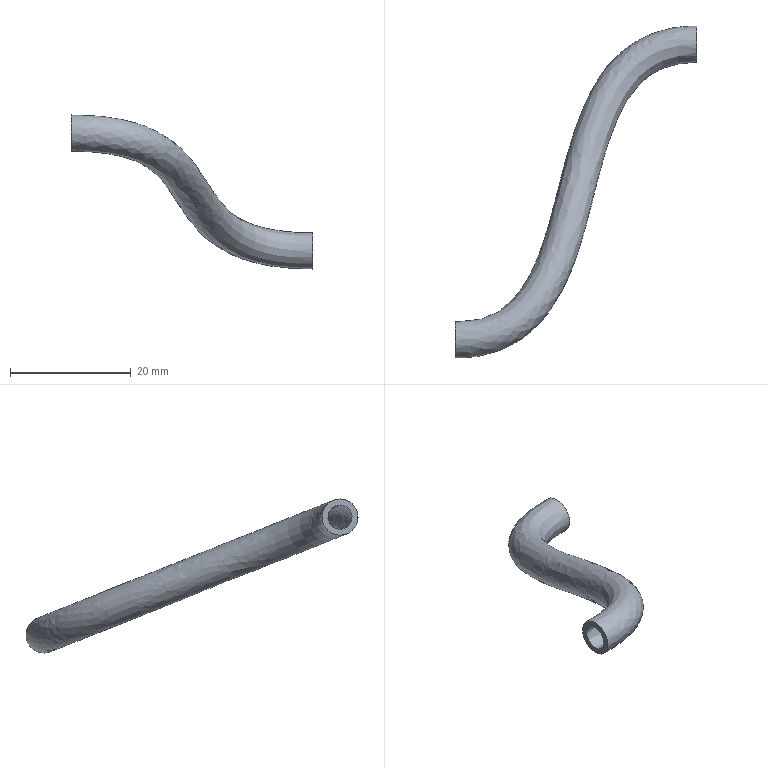Part | NX | features solid 2 | 1 solid | 4 faces | box 40.066 x 55.003 x 25.5 mm | volume 1141 mm3 | plane 2 | spline 2